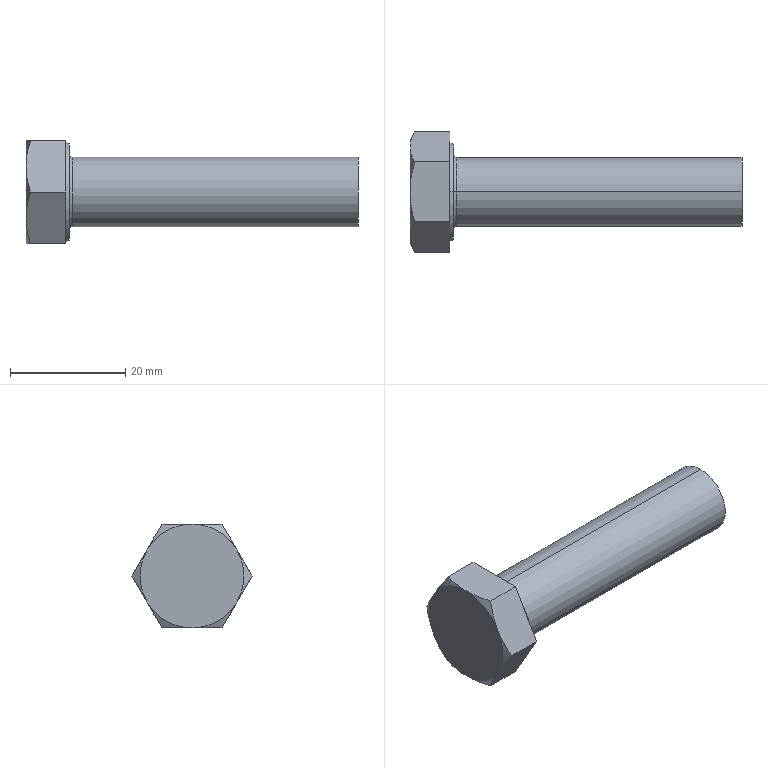Part | SolidWorks | features RevCut 3, Extrusion 1, Fillet 1, LPattern 1, Revolution 1 | 1 solid | 22 faces | box 57.5 x 20.785 x 18 mm | volume 7723 mm3 | plane 10 | cone 8 | torus 2 | cylinder 2 | commonest cylinder face diameters 12 x2
STEP:
#1=CARTESIAN_POINT('',(8.1,0.,6.));
#2=VERTEX_POINT('',#1);
#3=CARTESIAN_POINT('',(8.1,0.,-6.));
#4=VERTEX_POINT('',#3);
#5=CARTESIAN_POINT('',(8.1,0.,0.));
#6=DIRECTION('',(1.,0.,0.));
#7=DIRECTION('',(0.,0.,-1.));
#8=AXIS2_PLACEMENT_3D('',#5,#6,#7);
#9=CIRCLE('',#8,6.);
#10=EDGE_CURVE('',#2,#4,#9,.T.);
#11=ORIENTED_EDGE('',*,*,#10,.F.);
#12=CARTESIAN_POINT('',(7.5,0.,6.6));
#13=VERTEX_POINT('',#12);
#14=CARTESIAN_POINT('',(8.1,0.,6.6));
#15=DIRECTION('',(0.,1.,0.));
#16=DIRECTION('',(0.,0.,1.));
#17=AXIS2_PLACEMENT_3D('',#14,#15,#16);
#18=CIRCLE('',#17,0.6);
#19=EDGE_CURVE('',#2,#13,#18,.T.);
#20=ORIENTED_EDGE('',*,*,#19,.T.);
#21=CARTESIAN_POINT('',(7.5,0.,-6.6));
#22=VERTEX_POINT('',#21);
#23=CARTESIAN_POINT('',(7.5,0.,0.));
#24=DIRECTION('',(-1.,0.,0.));
#25=DIRECTION('',(0.,0.,-1.));
#26=AXIS2_PLACEMENT_3D('',#23,#24,#25);
#27=CIRCLE('',#26,6.6);
#28=EDGE_CURVE('',#22,#13,#27,.T.);
#29=ORIENTED_EDGE('',*,*,#28,.F.);
#30=CARTESIAN_POINT('',(8.1,0.,-6.6));
#31=DIRECTION('',(0.,-1.,0.));
#32=DIRECTION('',(0.,0.,-1.));
#33=AXIS2_PLACEMENT_3D('',#30,#31,#32);
#34=CIRCLE('',#33,0.6);
#35=EDGE_CURVE('',#4,#22,#34,.T.);
#36=ORIENTED_EDGE('',*,*,#35,.F.);
#37=EDGE_LOOP('',(#11,#20,#29,#36));
#38=FACE_OUTER_BOUND('',#37,.T.);
#39=CARTESIAN_POINT('',(8.1,0.,0.));
#40=DIRECTION('',(1.,0.,0.));
#41=DIRECTION('',(0.,0.,-1.));
#42=AXIS2_PLACEMENT_3D('',#39,#40,#41);
#43=TOROIDAL_SURFACE('',#42,6.6,0.6);
#44=ADVANCED_FACE('',(#38),#43,.F.);
#45=CARTESIAN_POINT('',(57.5,0.,6.));
#46=VERTEX_POINT('',#45);
#47=CARTESIAN_POINT('',(57.5,0.,-6.));
#48=VERTEX_POINT('',#47);
#49=CARTESIAN_POINT('',(57.5,0.,0.));
#50=DIRECTION('',(-1.,0.,0.));
#51=DIRECTION('',(0.,0.,1.));
#52=AXIS2_PLACEMENT_3D('',#49,#50,#51);
#53=CIRCLE('',#52,6.);
#54=EDGE_CURVE('',#46,#48,#53,.T.);
#55=ORIENTED_EDGE('',*,*,#54,.T.);
#56=CARTESIAN_POINT('',(0.,0.,-6.));
#57=DIRECTION('',(-1.,0.,0.));
#58=VECTOR('',#57,1000.);
#59=LINE('',#56,#58);
#60=EDGE_CURVE('',#48,#4,#59,.T.);
#61=ORIENTED_EDGE('',*,*,#60,.T.);
#62=CARTESIAN_POINT('',(8.1,0.,0.));
#63=DIRECTION('',(1.,0.,0.));
#64=DIRECTION('',(0.,0.,-1.));
#65=AXIS2_PLACEMENT_3D('',#62,#63,#64);
#66=CIRCLE('',#65,6.);
#67=EDGE_CURVE('',#4,#2,#66,.T.);
#68=ORIENTED_EDGE('',*,*,#67,.T.);
#69=CARTESIAN_POINT('',(0.,0.,6.));
#70=DIRECTION('',(-1.,0.,0.));
#71=VECTOR('',#70,1000.);
#72=LINE('',#69,#71);
#73=EDGE_CURVE('',#46,#2,#72,.T.);
#74=ORIENTED_EDGE('',*,*,#73,.F.);
#75=EDGE_LOOP('',(#55,#61,#68,#74));
#76=FACE_OUTER_BOUND('',#75,.T.);
#77=CARTESIAN_POINT('',(0.,0.,0.));
#78=DIRECTION('',(-1.,0.,0.));
#79=DIRECTION('',(0.,0.,1.));
#80=AXIS2_PLACEMENT_3D('',#77,#78,#79);
#81=CYLINDRICAL_SURFACE('',#80,6.);
#82=ADVANCED_FACE('',(#76),#81,.T.);
#83=CARTESIAN_POINT('',(7.5,0.,8.315));
#84=VERTEX_POINT('',#83);
#85=CARTESIAN_POINT('',(7.5,0.,-8.315));
#86=VERTEX_POINT('',#85);
#87=CARTESIAN_POINT('',(7.5,0.,0.));
#88=DIRECTION('',(-1.,0.,0.));
#89=DIRECTION('',(0.,0.,1.));
#90=AXIS2_PLACEMENT_3D('',#87,#88,#89);
#91=CIRCLE('',#90,8.315);
#92=EDGE_CURVE('',#84,#86,#91,.T.);
#93=ORIENTED_EDGE('',*,*,#92,.T.);
#94=CARTESIAN_POINT('',(6.9,0.,-8.661));
#95=VERTEX_POINT('',#94);
#96=CARTESIAN_POINT('',(6.9,0.,-8.661));
#97=DIRECTION('',(-0.866,0.,-0.5));
#98=VECTOR('',#97,1000.);
#99=LINE('',#96,#98);
#100=EDGE_CURVE('',#86,#95,#99,.T.);
#101=ORIENTED_EDGE('',*,*,#100,.T.);
#102=CARTESIAN_POINT('',(6.9,0.,8.661));
#103=VERTEX_POINT('',#102);
#104=CARTESIAN_POINT('',(6.9,0.,0.));
#105=DIRECTION('',(-1.,0.,0.));
#106=DIRECTION('',(0.,0.,1.));
#107=AXIS2_PLACEMENT_3D('',#104,#105,#106);
#108=CIRCLE('',#107,8.661);
#109=EDGE_CURVE('',#103,#95,#108,.T.);
#110=ORIENTED_EDGE('',*,*,#109,.F.);
#111=CARTESIAN_POINT('',(6.9,0.,8.661));
#112=DIRECTION('',(-0.866,0.,0.5));
#113=VECTOR('',#112,1000.);
#114=LINE('',#111,#113);
#115=EDGE_CURVE('',#84,#103,#114,.T.);
#116=ORIENTED_EDGE('',*,*,#115,.F.);
#117=EDGE_LOOP('',(#93,#101,#110,#116));
#118=FACE_OUTER_BOUND('',#117,.T.);
#119=CARTESIAN_POINT('',(6.9,0.,0.));
#120=DIRECTION('',(-1.,0.,0.));
#121=DIRECTION('',(0.,0.,1.));
#122=AXIS2_PLACEMENT_3D('',#119,#120,#121);
#123=CONICAL_SURFACE('',#122,8.661,0.5236);
#124=ADVANCED_FACE('',(#118),#123,.T.);
#125=CARTESIAN_POINT('',(6.9,5.196,-9.));
#126=VERTEX_POINT('',#125);
#127=CARTESIAN_POINT('',(6.9,10.392,0.));
#128=VERTEX_POINT('',#127);
#129=CARTESIAN_POINT('',(6.9,5.196,-9.));
#130=DIRECTION('',(0.,0.5,0.866));
#131=VECTOR('',#130,1000.);
#132=LINE('',#129,#131);
#133=EDGE_CURVE('',#126,#128,#132,.T.);
#134=ORIENTED_EDGE('',*,*,#133,.F.);
#135=CARTESIAN_POINT('',(0.8038,5.196,-9.));
#136=VERTEX_POINT('',#135);
#137=CARTESIAN_POINT('',(7.5,5.196,-9.));
#138=DIRECTION('',(-1.,0.,0.));
#139=VECTOR('',#138,1000.);
#140=LINE('',#137,#139);
#141=EDGE_CURVE('',#126,#136,#140,.T.);
#142=ORIENTED_EDGE('',*,*,#141,.T.);
#143=CARTESIAN_POINT('',(0.,7.794,-4.5));
#144=VERTEX_POINT('',#143);
#145=CARTESIAN_POINT('',(0.,7.794,-4.5));
#146=CARTESIAN_POINT('',(0.,7.574,-4.882));
#147=CARTESIAN_POINT('',(0.019,7.352,-5.266));
#148=CARTESIAN_POINT('',(0.09253,6.914,-6.024));
#149=CARTESIAN_POINT('',(0.147,6.697,-6.401));
#150=CARTESIAN_POINT('',(0.357,6.048,-7.525));
#151=CARTESIAN_POINT('',(0.5591,5.62,-8.266));
#152=CARTESIAN_POINT('',(0.8038,5.196,-9.));
#153=B_SPLINE_CURVE_WITH_KNOTS('',3,(#145,#146,#147,#148,#149,#150,#151,#152),.UNSPECIFIED.,.F.,.F.,(4,2,2,4),(0.005258,0.006567,0.007877,0.0105),.UNSPECIFIED.);
#154=EDGE_CURVE('',#144,#136,#153,.T.);
#155=ORIENTED_EDGE('',*,*,#154,.F.);
#156=CARTESIAN_POINT('',(0.8038,10.392,0.));
#157=VERTEX_POINT('',#156);
#158=CARTESIAN_POINT('',(0.8038,10.392,0.));
#159=CARTESIAN_POINT('',(0.5585,9.967,-0.7361));
#160=CARTESIAN_POINT('',(0.3563,9.539,-1.478));
#161=CARTESIAN_POINT('',(0.07661,8.674,-2.976));
#162=CARTESIAN_POINT('',(0.,8.237,-3.733));
#163=CARTESIAN_POINT('',(0.,7.794,-4.5));
#164=B_SPLINE_CURVE_WITH_KNOTS('',3,(#158,#159,#160,#161,#162,#163),.UNSPECIFIED.,.F.,.F.,(4,2,4),(0.000000238,0.002629,0.005258),.UNSPECIFIED.);
#165=EDGE_CURVE('',#157,#144,#164,.T.);
#166=ORIENTED_EDGE('',*,*,#165,.F.);
#167=CARTESIAN_POINT('',(7.5,10.392,0.));
#168=DIRECTION('',(-1.,0.,0.));
#169=VECTOR('',#168,1000.);
#170=LINE('',#167,#169);
#171=EDGE_CURVE('',#128,#157,#170,.T.);
#172=ORIENTED_EDGE('',*,*,#171,.F.);
#173=EDGE_LOOP('',(#134,#142,#155,#166,#172));
#174=FACE_OUTER_BOUND('',#173,.T.);
#175=CARTESIAN_POINT('',(7.5,5.196,-9.));
#176=DIRECTION('',(0.,-0.866,0.5));
#177=DIRECTION('',(0.,-0.5,-0.866));
#178=AXIS2_PLACEMENT_3D('',#175,#176,#177);
#179=PLANE('',#178);
#180=ADVANCED_FACE('',(#174),#179,.F.);
#181=CARTESIAN_POINT('',(6.9,5.196,9.));
#182=VERTEX_POINT('',#181);
#183=CARTESIAN_POINT('',(6.9,10.392,0.));
#184=DIRECTION('',(0.,-0.5,0.866));
#185=VECTOR('',#184,1000.);
#186=LINE('',#183,#185);
#187=EDGE_CURVE('',#128,#182,#186,.T.);
#188=ORIENTED_EDGE('',*,*,#187,.F.);
#189=ORIENTED_EDGE('',*,*,#171,.T.);
#190=CARTESIAN_POINT('',(0.,7.794,4.5));
#191=VERTEX_POINT('',#190);
#192=CARTESIAN_POINT('',(0.,7.794,4.5));
#193=CARTESIAN_POINT('',(0.,8.015,4.118));
#194=CARTESIAN_POINT('',(0.019,8.236,3.734));
#195=CARTESIAN_POINT('',(0.09253,8.674,2.976));
#196=CARTESIAN_POINT('',(0.147,8.892,2.599));
#197=CARTESIAN_POINT('',(0.357,9.541,1.475));
#198=CARTESIAN_POINT('',(0.5591,9.968,0.7343));
#199=CARTESIAN_POINT('',(0.8038,10.392,0.));
#200=B_SPLINE_CURVE_WITH_KNOTS('',3,(#192,#193,#194,#195,#196,#197,#198,#199),.UNSPECIFIED.,.F.,.F.,(4,2,2,4),(0.005258,0.006567,0.007877,0.0105),.UNSPECIFIED.);
#201=EDGE_CURVE('',#191,#157,#200,.T.);
#202=ORIENTED_EDGE('',*,*,#201,.F.);
#203=CARTESIAN_POINT('',(0.8038,5.196,9.));
#204=VERTEX_POINT('',#203);
#205=CARTESIAN_POINT('',(0.8038,5.196,9.));
#206=CARTESIAN_POINT('',(0.5585,5.621,8.264));
#207=CARTESIAN_POINT('',(0.3563,6.049,7.522));
#208=CARTESIAN_POINT('',(0.07661,6.914,6.024));
#209=CARTESIAN_POINT('',(0.,7.352,5.267));
#210=CARTESIAN_POINT('',(0.,7.794,4.5));
#211=B_SPLINE_CURVE_WITH_KNOTS('',3,(#205,#206,#207,#208,#209,#210),.UNSPECIFIED.,.F.,.F.,(4,2,4),(0.000000238,0.002629,0.005258),.UNSPECIFIED.);
#212=EDGE_CURVE('',#204,#191,#211,.T.);
#213=ORIENTED_EDGE('',*,*,#212,.F.);
#214=CARTESIAN_POINT('',(7.5,5.196,9.));
#215=DIRECTION('',(-1.,0.,0.));
#216=VECTOR('',#215,1000.);
#217=LINE('',#214,#216);
#218=EDGE_CURVE('',#182,#204,#217,.T.);
#219=ORIENTED_EDGE('',*,*,#218,.F.);
#220=EDGE_LOOP('',(#188,#189,#202,#213,#219));
#221=FACE_OUTER_BOUND('',#220,.T.);
#222=CARTESIAN_POINT('',(7.5,10.392,0.));
#223=DIRECTION('',(0.,-0.866,-0.5));
#224=DIRECTION('',(0.,0.5,-0.866));
#225=AXIS2_PLACEMENT_3D('',#222,#223,#224);
#226=PLANE('',#225);
#227=ADVANCED_FACE('',(#221),#226,.F.);
#228=CARTESIAN_POINT('',(6.9,-5.196,9.));
#229=VERTEX_POINT('',#228);
#230=CARTESIAN_POINT('',(6.9,5.196,9.));
#231=DIRECTION('',(0.,-1.,0.));
#232=VECTOR('',#231,1000.);
#233=LINE('',#230,#232);
#234=EDGE_CURVE('',#182,#229,#233,.T.);
#235=ORIENTED_EDGE('',*,*,#234,.F.);
#236=ORIENTED_EDGE('',*,*,#218,.T.);
#237=CARTESIAN_POINT('',(0.,0.,9.));
#238=VERTEX_POINT('',#237);
#239=CARTESIAN_POINT('',(0.,0.,9.));
#240=CARTESIAN_POINT('',(0.,0.4401,9.));
#241=CARTESIAN_POINT('',(0.01885,0.8832,9.));
#242=CARTESIAN_POINT('',(0.09319,1.767,9.));
#243=CARTESIAN_POINT('',(0.1482,2.204,9.));
#244=CARTESIAN_POINT('',(0.3593,3.505,9.));
#245=CARTESIAN_POINT('',(0.5612,4.356,9.));
#246=CARTESIAN_POINT('',(0.8038,5.196,9.));
#247=B_SPLINE_CURVE_WITH_KNOTS('',3,(#239,#240,#241,#242,#243,#244,#245,#246),.UNSPECIFIED.,.F.,.F.,(4,2,2,4),(0.01498,0.0163,0.01761,0.02025),.UNSPECIFIED.);
#248=EDGE_CURVE('',#238,#204,#247,.T.);
#249=ORIENTED_EDGE('',*,*,#248,.F.);
#250=CARTESIAN_POINT('',(0.8038,-5.196,9.));
#251=VERTEX_POINT('',#250);
#252=CARTESIAN_POINT('',(0.8038,-5.196,9.));
#253=CARTESIAN_POINT('',(0.5595,-4.35,9.));
#254=CARTESIAN_POINT('',(0.3552,-3.485,9.));
#255=CARTESIAN_POINT('',(0.07569,-1.752,9.));
#256=CARTESIAN_POINT('',(0.,-0.8794,9.));
#257=CARTESIAN_POINT('',(0.,0.,9.));
#258=B_SPLINE_CURVE_WITH_KNOTS('',3,(#252,#253,#254,#255,#256,#257),.UNSPECIFIED.,.F.,.F.,(4,2,4),(0.00972,0.01235,0.01498),.UNSPECIFIED.);
#259=EDGE_CURVE('',#251,#238,#258,.T.);
#260=ORIENTED_EDGE('',*,*,#259,.F.);
#261=CARTESIAN_POINT('',(7.5,-5.196,9.));
#262=DIRECTION('',(-1.,0.,0.));
#263=VECTOR('',#262,1000.);
#264=LINE('',#261,#263);
#265=EDGE_CURVE('',#229,#251,#264,.T.);
#266=ORIENTED_EDGE('',*,*,#265,.F.);
#267=EDGE_LOOP('',(#235,#236,#249,#260,#266));
#268=FACE_OUTER_BOUND('',#267,.T.);
#269=CARTESIAN_POINT('',(7.5,5.196,9.));
#270=DIRECTION('',(0.,0.,-1.));
#271=DIRECTION('',(-1.,0.,0.));
#272=AXIS2_PLACEMENT_3D('',#269,#270,#271);
#273=PLANE('',#272);
#274=ADVANCED_FACE('',(#268),#273,.F.);
#275=CARTESIAN_POINT('',(6.9,-10.392,0.));
#276=VERTEX_POINT('',#275);
#277=CARTESIAN_POINT('',(6.9,-10.392,0.));
#278=DIRECTION('',(0.,-0.5,-0.866));
#279=VECTOR('',#278,1000.);
#280=LINE('',#277,#279);
#281=EDGE_CURVE('',#229,#276,#280,.T.);
#282=ORIENTED_EDGE('',*,*,#281,.F.);
#283=ORIENTED_EDGE('',*,*,#265,.T.);
#284=CARTESIAN_POINT('',(0.,-7.794,4.5));
#285=VERTEX_POINT('',#284);
#286=CARTESIAN_POINT('',(0.,-7.794,4.5));
#287=CARTESIAN_POINT('',(0.,-7.574,4.882));
#288=CARTESIAN_POINT('',(0.019,-7.352,5.266));
#289=CARTESIAN_POINT('',(0.09253,-6.914,6.024));
#290=CARTESIAN_POINT('',(0.147,-6.697,6.401));
#291=CARTESIAN_POINT('',(0.357,-6.048,7.525));
#292=CARTESIAN_POINT('',(0.5591,-5.62,8.266));
#293=CARTESIAN_POINT('',(0.8038,-5.196,9.));
#294=B_SPLINE_CURVE_WITH_KNOTS('',3,(#286,#287,#288,#289,#290,#291,#292,#293),.UNSPECIFIED.,.F.,.F.,(4,2,2,4),(0.005258,0.006567,0.007877,0.0105),.UNSPECIFIED.);
#295=EDGE_CURVE('',#285,#251,#294,.T.);
#296=ORIENTED_EDGE('',*,*,#295,.F.);
#297=CARTESIAN_POINT('',(0.8038,-10.392,0.));
#298=VERTEX_POINT('',#297);
#299=CARTESIAN_POINT('',(0.8038,-10.392,0.));
#300=CARTESIAN_POINT('',(0.5585,-9.967,0.7361));
#301=CARTESIAN_POINT('',(0.3563,-9.539,1.478));
#302=CARTESIAN_POINT('',(0.07661,-8.674,2.976));
#303=CARTESIAN_POINT('',(0.,-8.237,3.733));
#304=CARTESIAN_POINT('',(0.,-7.794,4.5));
#305=B_SPLINE_CURVE_WITH_KNOTS('',3,(#299,#300,#301,#302,#303,#304),.UNSPECIFIED.,.F.,.F.,(4,2,4),(0.000000238,0.002629,0.005258),.UNSPECIFIED.);
#306=EDGE_CURVE('',#298,#285,#305,.T.);
#307=ORIENTED_EDGE('',*,*,#306,.F.);
#308=CARTESIAN_POINT('',(7.5,-10.392,0.));
#309=DIRECTION('',(-1.,0.,0.));
#310=VECTOR('',#309,1000.);
#311=LINE('',#308,#310);
#312=EDGE_CURVE('',#276,#298,#311,.T.);
#313=ORIENTED_EDGE('',*,*,#312,.F.);
#314=EDGE_LOOP('',(#282,#283,#296,#307,#313));
#315=FACE_OUTER_BOUND('',#314,.T.);
#316=CARTESIAN_POINT('',(7.5,-10.392,0.));
#317=DIRECTION('',(0.,0.866,-0.5));
#318=DIRECTION('',(0.,0.5,0.866));
#319=AXIS2_PLACEMENT_3D('',#316,#317,#318);
#320=PLANE('',#319);
#321=ADVANCED_FACE('',(#315),#320,.F.);
#322=CARTESIAN_POINT('',(6.9,-5.196,-9.));
#323=VERTEX_POINT('',#322);
#324=CARTESIAN_POINT('',(6.9,-5.196,-9.));
#325=DIRECTION('',(0.,0.5,-0.866));
#326=VECTOR('',#325,1000.);
#327=LINE('',#324,#326);
#328=EDGE_CURVE('',#276,#323,#327,.T.);
#329=ORIENTED_EDGE('',*,*,#328,.F.);
#330=ORIENTED_EDGE('',*,*,#312,.T.);
#331=CARTESIAN_POINT('',(0.,-7.794,-4.5));
#332=VERTEX_POINT('',#331);
#333=CARTESIAN_POINT('',(0.,-7.794,-4.5));
#334=CARTESIAN_POINT('',(0.,-8.015,-4.118));
#335=CARTESIAN_POINT('',(0.019,-8.236,-3.734));
#336=CARTESIAN_POINT('',(0.09253,-8.674,-2.976));
#337=CARTESIAN_POINT('',(0.147,-8.892,-2.599));
#338=CARTESIAN_POINT('',(0.357,-9.541,-1.475));
#339=CARTESIAN_POINT('',(0.5591,-9.968,-0.7343));
#340=CARTESIAN_POINT('',(0.8038,-10.392,0.));
#341=B_SPLINE_CURVE_WITH_KNOTS('',3,(#333,#334,#335,#336,#337,#338,#339,#340),.UNSPECIFIED.,.F.,.F.,(4,2,2,4),(0.005258,0.006567,0.007877,0.0105),.UNSPECIFIED.);
#342=EDGE_CURVE('',#332,#298,#341,.T.);
#343=ORIENTED_EDGE('',*,*,#342,.F.);
#344=CARTESIAN_POINT('',(0.8038,-5.196,-9.));
#345=VERTEX_POINT('',#344);
#346=CARTESIAN_POINT('',(0.8038,-5.196,-9.));
#347=CARTESIAN_POINT('',(0.5585,-5.621,-8.264));
#348=CARTESIAN_POINT('',(0.3563,-6.049,-7.522));
#349=CARTESIAN_POINT('',(0.07661,-6.914,-6.024));
#350=CARTESIAN_POINT('',(0.,-7.352,-5.267));
#351=CARTESIAN_POINT('',(0.,-7.794,-4.5));
#352=B_SPLINE_CURVE_WITH_KNOTS('',3,(#346,#347,#348,#349,#350,#351),.UNSPECIFIED.,.F.,.F.,(4,2,4),(0.000000238,0.002629,0.005258),.UNSPECIFIED.);
#353=EDGE_CURVE('',#345,#332,#352,.T.);
#354=ORIENTED_EDGE('',*,*,#353,.F.);
#355=CARTESIAN_POINT('',(7.5,-5.196,-9.));
#356=DIRECTION('',(-1.,0.,0.));
#357=VECTOR('',#356,1000.);
#358=LINE('',#355,#357);
#359=EDGE_CURVE('',#323,#345,#358,.T.);
#360=ORIENTED_EDGE('',*,*,#359,.F.);
#361=EDGE_LOOP('',(#329,#330,#343,#354,#360));
#362=FACE_OUTER_BOUND('',#361,.T.);
#363=CARTESIAN_POINT('',(7.5,-5.196,-9.));
#364=DIRECTION('',(0.,0.866,0.5));
#365=DIRECTION('',(0.,-0.5,0.866));
#366=AXIS2_PLACEMENT_3D('',#363,#364,#365);
#367=PLANE('',#366);
#368=ADVANCED_FACE('',(#362),#367,.F.);
#369=CARTESIAN_POINT('',(6.9,5.196,-9.));
#370=DIRECTION('',(0.,1.,0.));
#371=VECTOR('',#370,1000.);
#372=LINE('',#369,#371);
#373=EDGE_CURVE('',#323,#126,#372,.T.);
#374=ORIENTED_EDGE('',*,*,#373,.F.);
#375=ORIENTED_EDGE('',*,*,#359,.T.);
#376=CARTESIAN_POINT('',(0.,0.,-9.));
#377=VERTEX_POINT('',#376);
#378=CARTESIAN_POINT('',(0.,0.,-9.));
#379=CARTESIAN_POINT('',(0.,-0.8794,-9.));
#380=CARTESIAN_POINT('',(0.07569,-1.752,-9.));
#381=CARTESIAN_POINT('',(0.3552,-3.485,-9.));
#382=CARTESIAN_POINT('',(0.5595,-4.35,-9.));
#383=CARTESIAN_POINT('',(0.8038,-5.196,-9.));
#384=B_SPLINE_CURVE_WITH_KNOTS('',3,(#378,#379,#380,#381,#382,#383),.UNSPECIFIED.,.F.,.F.,(4,2,4),(0.03045,0.03308,0.03571),.UNSPECIFIED.);
#385=EDGE_CURVE('',#377,#345,#384,.T.);
#386=ORIENTED_EDGE('',*,*,#385,.F.);
#387=CARTESIAN_POINT('',(0.8038,5.196,-9.));
#388=CARTESIAN_POINT('',(0.5612,4.356,-9.));
#389=CARTESIAN_POINT('',(0.3593,3.505,-9.));
#390=CARTESIAN_POINT('',(0.1482,2.204,-9.));
#391=CARTESIAN_POINT('',(0.09319,1.767,-9.));
#392=CARTESIAN_POINT('',(0.01885,0.8832,-9.));
#393=CARTESIAN_POINT('',(0.,0.4401,-9.));
#394=CARTESIAN_POINT('',(0.,0.,-9.));
#395=B_SPLINE_CURVE_WITH_KNOTS('',3,(#387,#388,#389,#390,#391,#392,#393,#394),.UNSPECIFIED.,.F.,.F.,(4,2,2,4),(0.02519,0.02782,0.02914,0.03045),.UNSPECIFIED.);
#396=EDGE_CURVE('',#136,#377,#395,.T.);
#397=ORIENTED_EDGE('',*,*,#396,.F.);
#398=ORIENTED_EDGE('',*,*,#141,.F.);
#399=EDGE_LOOP('',(#374,#375,#386,#397,#398));
#400=FACE_OUTER_BOUND('',#399,.T.);
#401=CARTESIAN_POINT('',(7.5,5.196,-9.));
#402=DIRECTION('',(0.,0.,1.));
#403=DIRECTION('',(0.,-1.,0.));
#404=AXIS2_PLACEMENT_3D('',#401,#402,#403);
#405=PLANE('',#404);
#406=ADVANCED_FACE('',(#400),#405,.F.);
#407=ORIENTED_EDGE('',*,*,#353,.T.);
#408=CARTESIAN_POINT('',(0.,0.,0.));
#409=DIRECTION('',(1.,0.,0.));
#410=DIRECTION('',(0.,0.,-1.));
#411=AXIS2_PLACEMENT_3D('',#408,#409,#410);
#412=CIRCLE('',#411,9.);
#413=EDGE_CURVE('',#332,#377,#412,.T.);
#414=ORIENTED_EDGE('',*,*,#413,.T.);
#415=ORIENTED_EDGE('',*,*,#385,.T.);
#416=EDGE_LOOP('',(#407,#414,#415));
#417=FACE_OUTER_BOUND('',#416,.T.);
#418=CARTESIAN_POINT('',(0.,0.,0.));
#419=DIRECTION('',(1.,0.,0.));
#420=DIRECTION('',(0.,0.,-1.));
#421=AXIS2_PLACEMENT_3D('',#418,#419,#420);
#422=CONICAL_SURFACE('',#421,9.,1.047);
#423=ADVANCED_FACE('',(#417),#422,.T.);
#424=ORIENTED_EDGE('',*,*,#306,.T.);
#425=CARTESIAN_POINT('',(0.,0.,0.));
#426=DIRECTION('',(1.,0.,0.));
#427=DIRECTION('',(0.,0.,-1.));
#428=AXIS2_PLACEMENT_3D('',#425,#426,#427);
#429=CIRCLE('',#428,9.);
#430=EDGE_CURVE('',#285,#332,#429,.T.);
#431=ORIENTED_EDGE('',*,*,#430,.T.);
#432=ORIENTED_EDGE('',*,*,#342,.T.);
#433=EDGE_LOOP('',(#424,#431,#432));
#434=FACE_OUTER_BOUND('',#433,.T.);
#435=CARTESIAN_POINT('',(0.,0.,0.));
#436=DIRECTION('',(1.,0.,0.));
#437=DIRECTION('',(0.,0.,-1.));
#438=AXIS2_PLACEMENT_3D('',#435,#436,#437);
#439=CONICAL_SURFACE('',#438,9.,1.047);
#440=ADVANCED_FACE('',(#434),#439,.T.);
#441=ORIENTED_EDGE('',*,*,#259,.T.);
#442=CARTESIAN_POINT('',(0.,0.,0.));
#443=DIRECTION('',(1.,0.,0.));
#444=DIRECTION('',(0.,0.,-1.));
#445=AXIS2_PLACEMENT_3D('',#442,#443,#444);
#446=CIRCLE('',#445,9.);
#447=EDGE_CURVE('',#238,#285,#446,.T.);
#448=ORIENTED_EDGE('',*,*,#447,.T.);
#449=ORIENTED_EDGE('',*,*,#295,.T.);
#450=EDGE_LOOP('',(#441,#448,#449));
#451=FACE_OUTER_BOUND('',#450,.T.);
#452=CARTESIAN_POINT('',(0.,0.,0.));
#453=DIRECTION('',(1.,0.,0.));
#454=DIRECTION('',(0.,0.,-1.));
#455=AXIS2_PLACEMENT_3D('',#452,#453,#454);
#456=CONICAL_SURFACE('',#455,9.,1.047);
#457=ADVANCED_FACE('',(#451),#456,.T.);
#458=ORIENTED_EDGE('',*,*,#248,.T.);
#459=ORIENTED_EDGE('',*,*,#212,.T.);
#460=CARTESIAN_POINT('',(0.,0.,0.));
#461=DIRECTION('',(-1.,0.,0.));
#462=DIRECTION('',(0.,0.,1.));
#463=AXIS2_PLACEMENT_3D('',#460,#461,#462);
#464=CIRCLE('',#463,9.);
#465=EDGE_CURVE('',#238,#191,#464,.T.);
#466=ORIENTED_EDGE('',*,*,#465,.F.);
#467=EDGE_LOOP('',(#458,#459,#466));
#468=FACE_OUTER_BOUND('',#467,.T.);
#469=CARTESIAN_POINT('',(0.,0.,0.));
#470=DIRECTION('',(1.,0.,0.));
#471=DIRECTION('',(0.,0.,-1.));
#472=AXIS2_PLACEMENT_3D('',#469,#470,#471);
#473=CONICAL_SURFACE('',#472,9.,1.047);
#474=ADVANCED_FACE('',(#468),#473,.T.);
#475=ORIENTED_EDGE('',*,*,#201,.T.);
#476=ORIENTED_EDGE('',*,*,#165,.T.);
#477=CARTESIAN_POINT('',(0.,0.,0.));
#478=DIRECTION('',(1.,0.,0.));
#479=DIRECTION('',(0.,0.,-1.));
#480=AXIS2_PLACEMENT_3D('',#477,#478,#479);
#481=CIRCLE('',#480,9.);
#482=EDGE_CURVE('',#144,#191,#481,.T.);
#483=ORIENTED_EDGE('',*,*,#482,.T.);
#484=EDGE_LOOP('',(#475,#476,#483));
#485=FACE_OUTER_BOUND('',#484,.T.);
#486=CARTESIAN_POINT('',(0.,0.,0.));
#487=DIRECTION('',(1.,0.,0.));
#488=DIRECTION('',(0.,0.,-1.));
#489=AXIS2_PLACEMENT_3D('',#486,#487,#488);
#490=CONICAL_SURFACE('',#489,9.,1.047);
#491=ADVANCED_FACE('',(#485),#490,.T.);
#492=ORIENTED_EDGE('',*,*,#154,.T.);
#493=ORIENTED_EDGE('',*,*,#396,.T.);
#494=CARTESIAN_POINT('',(0.,0.,0.));
#495=DIRECTION('',(1.,0.,0.));
#496=DIRECTION('',(0.,0.,-1.));
#497=AXIS2_PLACEMENT_3D('',#494,#495,#496);
#498=CIRCLE('',#497,9.);
#499=EDGE_CURVE('',#377,#144,#498,.T.);
#500=ORIENTED_EDGE('',*,*,#499,.T.);
#501=EDGE_LOOP('',(#492,#493,#500));
#502=FACE_OUTER_BOUND('',#501,.T.);
#503=CARTESIAN_POINT('',(0.,0.,0.));
#504=DIRECTION('',(1.,0.,0.));
#505=DIRECTION('',(0.,0.,-1.));
#506=AXIS2_PLACEMENT_3D('',#503,#504,#505);
#507=CONICAL_SURFACE('',#506,9.,1.047);
#508=ADVANCED_FACE('',(#502),#507,.T.);
#509=ORIENTED_EDGE('',*,*,#499,.F.);
#510=ORIENTED_EDGE('',*,*,#413,.F.);
#511=ORIENTED_EDGE('',*,*,#430,.F.);
#512=ORIENTED_EDGE('',*,*,#447,.F.);
#513=ORIENTED_EDGE('',*,*,#465,.T.);
#514=ORIENTED_EDGE('',*,*,#482,.F.);
#515=EDGE_LOOP('',(#509,#510,#511,#512,#513,#514));
#516=FACE_OUTER_BOUND('',#515,.T.);
#517=CARTESIAN_POINT('',(0.,10.392,0.));
#518=DIRECTION('',(1.,0.,0.));
#519=DIRECTION('',(0.,0.,-1.));
#520=AXIS2_PLACEMENT_3D('',#517,#518,#519);
#521=PLANE('',#520);
#522=ADVANCED_FACE('',(#516),#521,.F.);
#523=ORIENTED_EDGE('',*,*,#109,.T.);
#524=CARTESIAN_POINT('',(6.9,0.,0.));
#525=DIRECTION('',(-1.,0.,0.));
#526=DIRECTION('',(0.,0.,1.));
#527=AXIS2_PLACEMENT_3D('',#524,#525,#526);
#528=CIRCLE('',#527,8.661);
#529=EDGE_CURVE('',#95,#103,#528,.T.);
#530=ORIENTED_EDGE('',*,*,#529,.T.);
#531=EDGE_LOOP('',(#523,#530));
#532=FACE_BOUND('',#531,.T.);
#533=ORIENTED_EDGE('',*,*,#133,.T.);
#534=ORIENTED_EDGE('',*,*,#187,.T.);
#535=ORIENTED_EDGE('',*,*,#234,.T.);
#536=ORIENTED_EDGE('',*,*,#281,.T.);
#537=ORIENTED_EDGE('',*,*,#328,.T.);
#538=ORIENTED_EDGE('',*,*,#373,.T.);
#539=EDGE_LOOP('',(#533,#534,#535,#536,#537,#538));
#540=FACE_OUTER_BOUND('',#539,.T.);
#541=CARTESIAN_POINT('',(6.9,8.661,0.));
#542=DIRECTION('',(1.,0.,0.));
#543=DIRECTION('',(0.,0.,-1.));
#544=AXIS2_PLACEMENT_3D('',#541,#542,#543);
#545=PLANE('',#544);
#546=ADVANCED_FACE('',(#532,#540),#545,.T.);
#547=ORIENTED_EDGE('',*,*,#100,.F.);
#548=CARTESIAN_POINT('',(7.5,0.,0.));
#549=DIRECTION('',(-1.,0.,0.));
#550=DIRECTION('',(0.,0.,1.));
#551=AXIS2_PLACEMENT_3D('',#548,#549,#550);
#552=CIRCLE('',#551,8.315);
#553=EDGE_CURVE('',#86,#84,#552,.T.);
#554=ORIENTED_EDGE('',*,*,#553,.T.);
#555=ORIENTED_EDGE('',*,*,#115,.T.);
#556=ORIENTED_EDGE('',*,*,#529,.F.);
#557=EDGE_LOOP('',(#547,#554,#555,#556));
#558=FACE_OUTER_BOUND('',#557,.T.);
#559=CARTESIAN_POINT('',(6.9,0.,0.));
#560=DIRECTION('',(-1.,0.,0.));
#561=DIRECTION('',(0.,0.,1.));
#562=AXIS2_PLACEMENT_3D('',#559,#560,#561);
#563=CONICAL_SURFACE('',#562,8.661,0.5236);
#564=ADVANCED_FACE('',(#558),#563,.T.);
#565=ORIENTED_EDGE('',*,*,#54,.F.);
#566=CARTESIAN_POINT('',(57.5,0.,0.));
#567=DIRECTION('',(-1.,0.,0.));
#568=DIRECTION('',(0.,0.,1.));
#569=AXIS2_PLACEMENT_3D('',#566,#567,#568);
#570=CIRCLE('',#569,6.);
#571=EDGE_CURVE('',#48,#46,#570,.T.);
#572=ORIENTED_EDGE('',*,*,#571,.F.);
#573=EDGE_LOOP('',(#565,#572));
#574=FACE_OUTER_BOUND('',#573,.T.);
#575=CARTESIAN_POINT('',(57.5,0.,0.));
#576=DIRECTION('',(-1.,0.,0.));
#577=DIRECTION('',(0.,0.,1.));
#578=AXIS2_PLACEMENT_3D('',#575,#576,#577);
#579=PLANE('',#578);
#580=ADVANCED_FACE('',(#574),#579,.F.);
#581=ORIENTED_EDGE('',*,*,#60,.F.);
#582=ORIENTED_EDGE('',*,*,#571,.T.);
#583=ORIENTED_EDGE('',*,*,#73,.T.);
#584=ORIENTED_EDGE('',*,*,#10,.T.);
#585=EDGE_LOOP('',(#581,#582,#583,#584));
#586=FACE_OUTER_BOUND('',#585,.T.);
#587=CARTESIAN_POINT('',(0.,0.,0.));
#588=DIRECTION('',(-1.,0.,0.));
#589=DIRECTION('',(0.,0.,1.));
#590=AXIS2_PLACEMENT_3D('',#587,#588,#589);
#591=CYLINDRICAL_SURFACE('',#590,6.);
#592=ADVANCED_FACE('',(#586),#591,.T.);
#593=ORIENTED_EDGE('',*,*,#28,.T.);
#594=CARTESIAN_POINT('',(7.5,0.,0.));
#595=DIRECTION('',(-1.,0.,0.));
#596=DIRECTION('',(0.,0.,-1.));
#597=AXIS2_PLACEMENT_3D('',#594,#595,#596);
#598=CIRCLE('',#597,6.6);
#599=EDGE_CURVE('',#13,#22,#598,.T.);
#600=ORIENTED_EDGE('',*,*,#599,.T.);
#601=EDGE_LOOP('',(#593,#600));
#602=FACE_BOUND('',#601,.T.);
#603=ORIENTED_EDGE('',*,*,#92,.F.);
#604=ORIENTED_EDGE('',*,*,#553,.F.);
#605=EDGE_LOOP('',(#603,#604));
#606=FACE_OUTER_BOUND('',#605,.T.);
#607=CARTESIAN_POINT('',(7.5,10.392,0.));
#608=DIRECTION('',(1.,0.,0.));
#609=DIRECTION('',(0.,0.,-1.));
#610=AXIS2_PLACEMENT_3D('',#607,#608,#609);
#611=PLANE('',#610);
#612=ADVANCED_FACE('',(#602,#606),#611,.T.);
#613=ORIENTED_EDGE('',*,*,#19,.F.);
#614=ORIENTED_EDGE('',*,*,#67,.F.);
#615=ORIENTED_EDGE('',*,*,#35,.T.);
#616=ORIENTED_EDGE('',*,*,#599,.F.);
#617=EDGE_LOOP('',(#613,#614,#615,#616));
#618=FACE_OUTER_BOUND('',#617,.T.);
#619=CARTESIAN_POINT('',(8.1,0.,0.));
#620=DIRECTION('',(1.,0.,0.));
#621=DIRECTION('',(0.,0.,-1.));
#622=AXIS2_PLACEMENT_3D('',#619,#620,#621);
#623=TOROIDAL_SURFACE('',#622,6.6,0.6);
#624=ADVANCED_FACE('',(#618),#623,.F.);
#625=CLOSED_SHELL('',(#44,#82,#124,#180,#227,#274,#321,#368,#406,#423,#440,#457,#474,#491,#508,#522,#546,#564,#580,#592,#612,#624));
#626=MANIFOLD_SOLID_BREP('',#625);
#627=CARTESIAN_POINT('',(0.,0.,0.));
#628=DIRECTION('',(0.,0.,1.));
#629=DIRECTION('',(1.,0.,0.));
#630=AXIS2_PLACEMENT_3D('',#627,#628,#629);
#631=(LENGTH_UNIT()NAMED_UNIT(*)SI_UNIT(.MILLI.,.METRE.));
#632=UNCERTAINTY_MEASURE_WITH_UNIT(LENGTH_MEASURE(0.00001),#631,'','');
#633=(NAMED_UNIT(*)PLANE_ANGLE_UNIT()SI_UNIT($,.RADIAN.));
#634=(NAMED_UNIT(*)SI_UNIT($,.STERADIAN.)SOLID_ANGLE_UNIT());
#635=(GEOMETRIC_REPRESENTATION_CONTEXT(3)GLOBAL_UNCERTAINTY_ASSIGNED_CONTEXT((#632))GLOBAL_UNIT_ASSIGNED_CONTEXT((#631,#633,#634))REPRESENTATION_CONTEXT('',''));
#636=ADVANCED_BREP_SHAPE_REPRESENTATION('',(#626,#630),#635);